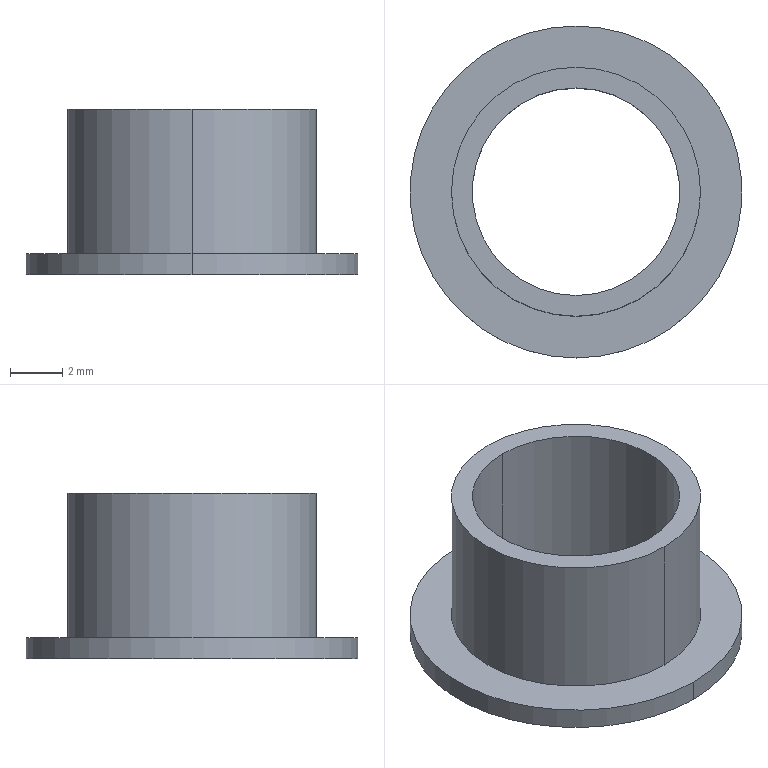Part | NX | features BREP 1 | 1 solid | 9 faces | box 12.7 x 12.7 x 6.35 mm | volume 183.302 mm3 | cylinder 6 | plane 3 | commonest cylinder face diameters 7.938 x2 9.525 x2 12.7 x2
STEP:
#1=CARTESIAN_POINT('',(0.,3.969,6.35));
#2=VERTEX_POINT('',#1);
#3=CARTESIAN_POINT('',(0.,-3.969,6.35));
#4=VERTEX_POINT('',#3);
#5=CARTESIAN_POINT('',(0.,0.,6.35));
#6=DIRECTION('',(0.,0.,1.));
#7=DIRECTION('',(0.,1.,0.));
#8=AXIS2_PLACEMENT_3D('',#5,#6,#7);
#9=CIRCLE('',#8,3.969);
#10=EDGE_CURVE('',#2,#4,#9,.T.);
#11=ORIENTED_EDGE('',*,*,#10,.T.);
#12=CARTESIAN_POINT('',(0.,-3.969,0.));
#13=VERTEX_POINT('',#12);
#14=CARTESIAN_POINT('',(0.,-3.969,0.));
#15=DIRECTION('',(0.,0.,1.));
#16=VECTOR('',#15,1000.);
#17=LINE('',#14,#16);
#18=EDGE_CURVE('',#4,#13,#17,.F.);
#19=ORIENTED_EDGE('',*,*,#18,.T.);
#20=CARTESIAN_POINT('',(0.,3.969,0.));
#21=VERTEX_POINT('',#20);
#22=CARTESIAN_POINT('',(0.,0.,0.));
#23=DIRECTION('',(0.,0.,1.));
#24=DIRECTION('',(0.,1.,0.));
#25=AXIS2_PLACEMENT_3D('',#22,#23,#24);
#26=CIRCLE('',#25,3.969);
#27=EDGE_CURVE('',#21,#13,#26,.T.);
#28=ORIENTED_EDGE('',*,*,#27,.F.);
#29=CARTESIAN_POINT('',(0.,3.969,0.));
#30=DIRECTION('',(0.,0.,1.));
#31=VECTOR('',#30,1000.);
#32=LINE('',#29,#31);
#33=EDGE_CURVE('',#2,#21,#32,.F.);
#34=ORIENTED_EDGE('',*,*,#33,.F.);
#35=EDGE_LOOP('',(#11,#19,#28,#34));
#36=FACE_BOUND('',#35,.T.);
#37=CARTESIAN_POINT('',(0.,0.,-0.3175));
#38=DIRECTION('',(0.,0.,1.));
#39=DIRECTION('',(0.,-1.,0.));
#40=AXIS2_PLACEMENT_3D('',#37,#38,#39);
#41=CYLINDRICAL_SURFACE('',#40,3.969);
#42=ADVANCED_FACE('',(#36),#41,.F.);
#43=CARTESIAN_POINT('',(0.,0.,0.));
#44=DIRECTION('',(0.,0.,-1.));
#45=DIRECTION('',(0.,1.,0.));
#46=AXIS2_PLACEMENT_3D('',#43,#44,#45);
#47=CIRCLE('',#46,3.969);
#48=EDGE_CURVE('',#21,#13,#47,.T.);
#49=ORIENTED_EDGE('',*,*,#48,.T.);
#50=ORIENTED_EDGE('',*,*,#18,.F.);
#51=CARTESIAN_POINT('',(0.,0.,6.35));
#52=DIRECTION('',(0.,0.,-1.));
#53=DIRECTION('',(0.,1.,0.));
#54=AXIS2_PLACEMENT_3D('',#51,#52,#53);
#55=CIRCLE('',#54,3.969);
#56=EDGE_CURVE('',#2,#4,#55,.T.);
#57=ORIENTED_EDGE('',*,*,#56,.F.);
#58=ORIENTED_EDGE('',*,*,#33,.T.);
#59=EDGE_LOOP('',(#49,#50,#57,#58));
#60=FACE_BOUND('',#59,.T.);
#61=CARTESIAN_POINT('',(0.,0.,-0.3175));
#62=DIRECTION('',(0.,0.,1.));
#63=DIRECTION('',(0.,-1.,0.));
#64=AXIS2_PLACEMENT_3D('',#61,#62,#63);
#65=CYLINDRICAL_SURFACE('',#64,3.969);
#66=ADVANCED_FACE('',(#60),#65,.F.);
#67=CARTESIAN_POINT('',(0.,4.763,6.35));
#68=VERTEX_POINT('',#67);
#69=CARTESIAN_POINT('',(0.,-4.763,6.35));
#70=VERTEX_POINT('',#69);
#71=CARTESIAN_POINT('',(0.,0.,6.35));
#72=DIRECTION('',(0.,0.,-1.));
#73=DIRECTION('',(0.,1.,0.));
#74=AXIS2_PLACEMENT_3D('',#71,#72,#73);
#75=CIRCLE('',#74,4.763);
#76=EDGE_CURVE('',#68,#70,#75,.T.);
#77=ORIENTED_EDGE('',*,*,#76,.F.);
#78=CARTESIAN_POINT('',(0.,0.,6.35));
#79=DIRECTION('',(0.,0.,1.));
#80=DIRECTION('',(0.,1.,0.));
#81=AXIS2_PLACEMENT_3D('',#78,#79,#80);
#82=CIRCLE('',#81,4.763);
#83=EDGE_CURVE('',#68,#70,#82,.T.);
#84=ORIENTED_EDGE('',*,*,#83,.T.);
#85=EDGE_LOOP('',(#77,#84));
#86=FACE_BOUND('',#85,.T.);
#87=ORIENTED_EDGE('',*,*,#10,.F.);
#88=ORIENTED_EDGE('',*,*,#56,.T.);
#89=EDGE_LOOP('',(#87,#88));
#90=FACE_BOUND('',#89,.T.);
#91=CARTESIAN_POINT('',(0.,0.,6.35));
#92=DIRECTION('',(0.,0.,1.));
#93=DIRECTION('',(1.,0.,0.));
#94=AXIS2_PLACEMENT_3D('',#91,#92,#93);
#95=PLANE('',#94);
#96=ADVANCED_FACE('',(#86,#90),#95,.T.);
#97=CARTESIAN_POINT('',(0.,4.763,0.8128));
#98=VERTEX_POINT('',#97);
#99=CARTESIAN_POINT('',(0.,-4.763,0.8128));
#100=VERTEX_POINT('',#99);
#101=CARTESIAN_POINT('',(0.,0.,0.8128));
#102=DIRECTION('',(0.,0.,1.));
#103=DIRECTION('',(0.,1.,0.));
#104=AXIS2_PLACEMENT_3D('',#101,#102,#103);
#105=CIRCLE('',#104,4.763);
#106=EDGE_CURVE('',#98,#100,#105,.T.);
#107=ORIENTED_EDGE('',*,*,#106,.T.);
#108=CARTESIAN_POINT('',(0.,-4.763,6.35));
#109=DIRECTION('',(0.,0.,-1.));
#110=VECTOR('',#109,1000.);
#111=LINE('',#108,#110);
#112=EDGE_CURVE('',#100,#70,#111,.F.);
#113=ORIENTED_EDGE('',*,*,#112,.T.);
#114=ORIENTED_EDGE('',*,*,#83,.F.);
#115=CARTESIAN_POINT('',(0.,4.763,6.35));
#116=DIRECTION('',(0.,0.,-1.));
#117=VECTOR('',#116,1000.);
#118=LINE('',#115,#117);
#119=EDGE_CURVE('',#98,#68,#118,.F.);
#120=ORIENTED_EDGE('',*,*,#119,.F.);
#121=EDGE_LOOP('',(#107,#113,#114,#120));
#122=FACE_BOUND('',#121,.T.);
#123=CARTESIAN_POINT('',(0.,0.,-0.3175));
#124=DIRECTION('',(0.,0.,1.));
#125=DIRECTION('',(0.,-1.,0.));
#126=AXIS2_PLACEMENT_3D('',#123,#124,#125);
#127=CYLINDRICAL_SURFACE('',#126,4.763);
#128=ADVANCED_FACE('',(#122),#127,.T.);
#129=ORIENTED_EDGE('',*,*,#76,.T.);
#130=ORIENTED_EDGE('',*,*,#112,.F.);
#131=CARTESIAN_POINT('',(0.,0.,0.8128));
#132=DIRECTION('',(0.,0.,-1.));
#133=DIRECTION('',(0.,1.,0.));
#134=AXIS2_PLACEMENT_3D('',#131,#132,#133);
#135=CIRCLE('',#134,4.763);
#136=EDGE_CURVE('',#98,#100,#135,.T.);
#137=ORIENTED_EDGE('',*,*,#136,.F.);
#138=ORIENTED_EDGE('',*,*,#119,.T.);
#139=EDGE_LOOP('',(#129,#130,#137,#138));
#140=FACE_BOUND('',#139,.T.);
#141=CARTESIAN_POINT('',(0.,0.,-0.3175));
#142=DIRECTION('',(0.,0.,1.));
#143=DIRECTION('',(0.,-1.,0.));
#144=AXIS2_PLACEMENT_3D('',#141,#142,#143);
#145=CYLINDRICAL_SURFACE('',#144,4.763);
#146=ADVANCED_FACE('',(#140),#145,.T.);
#147=CARTESIAN_POINT('',(0.,6.35,0.8128));
#148=VERTEX_POINT('',#147);
#149=CARTESIAN_POINT('',(0.,-6.35,0.8128));
#150=VERTEX_POINT('',#149);
#151=CARTESIAN_POINT('',(0.,0.,0.8128));
#152=DIRECTION('',(0.,0.,-1.));
#153=DIRECTION('',(0.,1.,0.));
#154=AXIS2_PLACEMENT_3D('',#151,#152,#153);
#155=CIRCLE('',#154,6.35);
#156=EDGE_CURVE('',#148,#150,#155,.T.);
#157=ORIENTED_EDGE('',*,*,#156,.F.);
#158=CARTESIAN_POINT('',(0.,0.,0.8128));
#159=DIRECTION('',(0.,0.,1.));
#160=DIRECTION('',(0.,1.,0.));
#161=AXIS2_PLACEMENT_3D('',#158,#159,#160);
#162=CIRCLE('',#161,6.35);
#163=EDGE_CURVE('',#148,#150,#162,.T.);
#164=ORIENTED_EDGE('',*,*,#163,.T.);
#165=EDGE_LOOP('',(#157,#164));
#166=FACE_BOUND('',#165,.T.);
#167=ORIENTED_EDGE('',*,*,#106,.F.);
#168=ORIENTED_EDGE('',*,*,#136,.T.);
#169=EDGE_LOOP('',(#167,#168));
#170=FACE_BOUND('',#169,.T.);
#171=CARTESIAN_POINT('',(0.,0.,0.8128));
#172=DIRECTION('',(0.,0.,1.));
#173=DIRECTION('',(1.,0.,0.));
#174=AXIS2_PLACEMENT_3D('',#171,#172,#173);
#175=PLANE('',#174);
#176=ADVANCED_FACE('',(#166,#170),#175,.T.);
#177=CARTESIAN_POINT('',(0.,6.35,0.));
#178=VERTEX_POINT('',#177);
#179=CARTESIAN_POINT('',(0.,-6.35,0.));
#180=VERTEX_POINT('',#179);
#181=CARTESIAN_POINT('',(0.,0.,0.));
#182=DIRECTION('',(0.,0.,1.));
#183=DIRECTION('',(0.,1.,0.));
#184=AXIS2_PLACEMENT_3D('',#181,#182,#183);
#185=CIRCLE('',#184,6.35);
#186=EDGE_CURVE('',#178,#180,#185,.T.);
#187=ORIENTED_EDGE('',*,*,#186,.T.);
#188=CARTESIAN_POINT('',(0.,-6.35,0.8128));
#189=DIRECTION('',(0.,0.,-1.));
#190=VECTOR('',#189,1000.);
#191=LINE('',#188,#190);
#192=EDGE_CURVE('',#180,#150,#191,.F.);
#193=ORIENTED_EDGE('',*,*,#192,.T.);
#194=ORIENTED_EDGE('',*,*,#163,.F.);
#195=CARTESIAN_POINT('',(0.,6.35,0.8128));
#196=DIRECTION('',(0.,0.,-1.));
#197=VECTOR('',#196,1000.);
#198=LINE('',#195,#197);
#199=EDGE_CURVE('',#178,#148,#198,.F.);
#200=ORIENTED_EDGE('',*,*,#199,.F.);
#201=EDGE_LOOP('',(#187,#193,#194,#200));
#202=FACE_BOUND('',#201,.T.);
#203=CARTESIAN_POINT('',(0.,0.,-0.3175));
#204=DIRECTION('',(0.,0.,1.));
#205=DIRECTION('',(0.,-1.,0.));
#206=AXIS2_PLACEMENT_3D('',#203,#204,#205);
#207=CYLINDRICAL_SURFACE('',#206,6.35);
#208=ADVANCED_FACE('',(#202),#207,.T.);
#209=ORIENTED_EDGE('',*,*,#156,.T.);
#210=ORIENTED_EDGE('',*,*,#192,.F.);
#211=CARTESIAN_POINT('',(0.,0.,0.));
#212=DIRECTION('',(0.,0.,-1.));
#213=DIRECTION('',(0.,1.,0.));
#214=AXIS2_PLACEMENT_3D('',#211,#212,#213);
#215=CIRCLE('',#214,6.35);
#216=EDGE_CURVE('',#178,#180,#215,.T.);
#217=ORIENTED_EDGE('',*,*,#216,.F.);
#218=ORIENTED_EDGE('',*,*,#199,.T.);
#219=EDGE_LOOP('',(#209,#210,#217,#218));
#220=FACE_BOUND('',#219,.T.);
#221=CARTESIAN_POINT('',(0.,0.,-0.3175));
#222=DIRECTION('',(0.,0.,1.));
#223=DIRECTION('',(0.,-1.,0.));
#224=AXIS2_PLACEMENT_3D('',#221,#222,#223);
#225=CYLINDRICAL_SURFACE('',#224,6.35);
#226=ADVANCED_FACE('',(#220),#225,.T.);
#227=ORIENTED_EDGE('',*,*,#186,.F.);
#228=ORIENTED_EDGE('',*,*,#216,.T.);
#229=EDGE_LOOP('',(#227,#228));
#230=FACE_BOUND('',#229,.T.);
#231=ORIENTED_EDGE('',*,*,#48,.F.);
#232=ORIENTED_EDGE('',*,*,#27,.T.);
#233=EDGE_LOOP('',(#231,#232));
#234=FACE_BOUND('',#233,.T.);
#235=CARTESIAN_POINT('',(0.,0.,0.));
#236=DIRECTION('',(0.,0.,1.));
#237=DIRECTION('',(1.,0.,0.));
#238=AXIS2_PLACEMENT_3D('',#235,#236,#237);
#239=PLANE('',#238);
#240=ADVANCED_FACE('',(#230,#234),#239,.F.);
#241=CLOSED_SHELL('',(#42,#66,#96,#128,#146,#176,#208,#226,#240));
#242=MANIFOLD_SOLID_BREP('',#241);
#243=(LENGTH_UNIT()NAMED_UNIT(*)SI_UNIT(.MILLI.,.METRE.));
#244=UNCERTAINTY_MEASURE_WITH_UNIT(LENGTH_MEASURE(0.00001),#243,'','');
#245=(NAMED_UNIT(*)PLANE_ANGLE_UNIT()SI_UNIT($,.RADIAN.));
#246=(NAMED_UNIT(*)SI_UNIT($,.STERADIAN.)SOLID_ANGLE_UNIT());
#247=(GEOMETRIC_REPRESENTATION_CONTEXT(3)GLOBAL_UNCERTAINTY_ASSIGNED_CONTEXT((#244))GLOBAL_UNIT_ASSIGNED_CONTEXT((#243,#245,#246))REPRESENTATION_CONTEXT('',''));
#248=ADVANCED_BREP_SHAPE_REPRESENTATION('',(#242),#247);